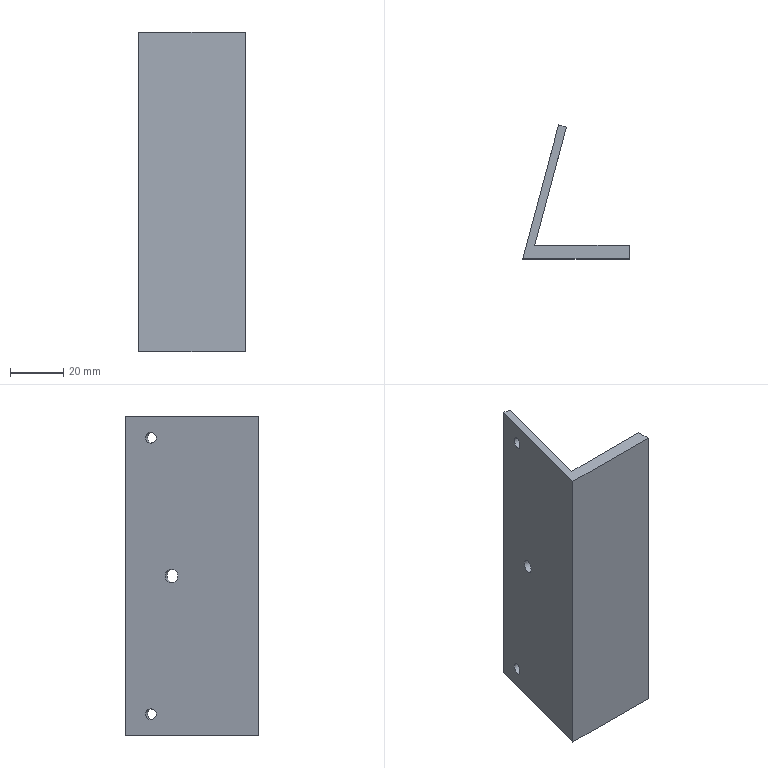Part | NX | features DATUM_CSYS 5, SKETCH 4, EXTRUDE 3, OFFSET_REGION 1 | 1 solid | 11 faces | box 40 x 50.228 x 120 mm | volume 40168 mm3 | plane 8 | cylinder 3 | commonest cylinder face diameters 4.2 x2 5 x1
STEP:
#1=CARTESIAN_POINT('',(0.,0.,-60.));
#2=VERTEX_POINT('',#1);
#3=CARTESIAN_POINT('',(40.,0.,-60.));
#4=VERTEX_POINT('',#3);
#5=CARTESIAN_POINT('',(5.176,0.,-60.));
#6=DIRECTION('',(1.,0.,0.));
#7=VECTOR('',#6,1000.);
#8=LINE('',#5,#7);
#9=EDGE_CURVE('',#2,#4,#8,.T.);
#10=ORIENTED_EDGE('',*,*,#9,.T.);
#11=CARTESIAN_POINT('',(40.,0.,60.));
#12=VERTEX_POINT('',#11);
#13=CARTESIAN_POINT('',(40.,0.,60.));
#14=DIRECTION('',(0.,0.,-1.));
#15=VECTOR('',#14,1000.);
#16=LINE('',#13,#15);
#17=EDGE_CURVE('',#12,#4,#16,.T.);
#18=ORIENTED_EDGE('',*,*,#17,.F.);
#19=CARTESIAN_POINT('',(0.,0.,60.));
#20=VERTEX_POINT('',#19);
#21=CARTESIAN_POINT('',(0.,0.,60.));
#22=DIRECTION('',(1.,0.,0.));
#23=VECTOR('',#22,1000.);
#24=LINE('',#21,#23);
#25=EDGE_CURVE('',#20,#12,#24,.T.);
#26=ORIENTED_EDGE('',*,*,#25,.F.);
#27=CARTESIAN_POINT('',(0.,0.,60.));
#28=DIRECTION('',(0.,0.,-1.));
#29=VECTOR('',#28,1000.);
#30=LINE('',#27,#29);
#31=EDGE_CURVE('',#20,#2,#30,.T.);
#32=ORIENTED_EDGE('',*,*,#31,.T.);
#33=EDGE_LOOP('',(#10,#18,#26,#32));
#34=FACE_BOUND('',#33,.T.);
#35=CARTESIAN_POINT('',(5.176,0.,60.));
#36=DIRECTION('',(0.,1.,0.));
#37=DIRECTION('',(0.,0.,1.));
#38=AXIS2_PLACEMENT_3D('',#35,#36,#37);
#39=PLANE('',#38);
#40=ADVANCED_FACE('',(#34),#39,.F.);
#41=CARTESIAN_POINT('',(40.,5.,-60.));
#42=VERTEX_POINT('',#41);
#43=CARTESIAN_POINT('',(40.,0.,-60.));
#44=DIRECTION('',(0.,1.,0.));
#45=VECTOR('',#44,1000.);
#46=LINE('',#43,#45);
#47=EDGE_CURVE('',#4,#42,#46,.T.);
#48=ORIENTED_EDGE('',*,*,#47,.T.);
#49=CARTESIAN_POINT('',(40.,5.,60.));
#50=VERTEX_POINT('',#49);
#51=CARTESIAN_POINT('',(40.,5.,60.));
#52=DIRECTION('',(0.,0.,-1.));
#53=VECTOR('',#52,1000.);
#54=LINE('',#51,#53);
#55=EDGE_CURVE('',#50,#42,#54,.T.);
#56=ORIENTED_EDGE('',*,*,#55,.F.);
#57=CARTESIAN_POINT('',(40.,0.,60.));
#58=DIRECTION('',(0.,1.,0.));
#59=VECTOR('',#58,1000.);
#60=LINE('',#57,#59);
#61=EDGE_CURVE('',#12,#50,#60,.T.);
#62=ORIENTED_EDGE('',*,*,#61,.F.);
#63=ORIENTED_EDGE('',*,*,#17,.T.);
#64=EDGE_LOOP('',(#48,#56,#62,#63));
#65=FACE_BOUND('',#64,.T.);
#66=CARTESIAN_POINT('',(40.,0.,60.));
#67=DIRECTION('',(-1.,0.,0.));
#68=DIRECTION('',(0.,0.,1.));
#69=AXIS2_PLACEMENT_3D('',#66,#67,#68);
#70=PLANE('',#69);
#71=ADVANCED_FACE('',(#65),#70,.F.);
#72=CARTESIAN_POINT('',(4.446,5.,-60.));
#73=VERTEX_POINT('',#72);
#74=CARTESIAN_POINT('',(40.,5.,-60.));
#75=DIRECTION('',(-1.,0.,0.));
#76=VECTOR('',#75,1000.);
#77=LINE('',#74,#76);
#78=EDGE_CURVE('',#42,#73,#77,.T.);
#79=ORIENTED_EDGE('',*,*,#78,.T.);
#80=CARTESIAN_POINT('',(4.446,5.,60.));
#81=VERTEX_POINT('',#80);
#82=CARTESIAN_POINT('',(4.446,5.,60.));
#83=DIRECTION('',(0.,0.,-1.));
#84=VECTOR('',#83,1000.);
#85=LINE('',#82,#84);
#86=EDGE_CURVE('',#81,#73,#85,.T.);
#87=ORIENTED_EDGE('',*,*,#86,.F.);
#88=CARTESIAN_POINT('',(40.,5.,60.));
#89=DIRECTION('',(-1.,0.,0.));
#90=VECTOR('',#89,1000.);
#91=LINE('',#88,#90);
#92=EDGE_CURVE('',#50,#81,#91,.T.);
#93=ORIENTED_EDGE('',*,*,#92,.F.);
#94=ORIENTED_EDGE('',*,*,#55,.T.);
#95=EDGE_LOOP('',(#79,#87,#93,#94));
#96=FACE_BOUND('',#95,.T.);
#97=CARTESIAN_POINT('',(40.,5.,60.));
#98=DIRECTION('',(0.,-1.,0.));
#99=DIRECTION('',(0.,0.,-1.));
#100=AXIS2_PLACEMENT_3D('',#97,#98,#99);
#101=PLANE('',#100);
#102=ADVANCED_FACE('',(#96),#101,.F.);
#103=CARTESIAN_POINT('',(11.051,29.65,0.));
#104=VERTEX_POINT('',#103);
#105=CARTESIAN_POINT('',(11.698,32.065,0.));
#106=DIRECTION('',(-0.9659,0.2588,0.));
#107=DIRECTION('',(-0.2588,-0.9659,0.));
#108=AXIS2_PLACEMENT_3D('',#105,#106,#107);
#109=CIRCLE('',#108,2.5);
#110=EDGE_CURVE('',#104,#104,#109,.F.);
#111=ORIENTED_EDGE('',*,*,#110,.F.);
#112=EDGE_LOOP('',(#111));
#113=FACE_BOUND('',#112,.T.);
#114=CARTESIAN_POINT('',(13.225,37.764,-52.));
#115=VERTEX_POINT('',#114);
#116=CARTESIAN_POINT('',(13.768,39.792,-52.));
#117=DIRECTION('',(-0.9659,0.2588,0.));
#118=DIRECTION('',(-0.2588,-0.9659,0.));
#119=AXIS2_PLACEMENT_3D('',#116,#117,#118);
#120=CIRCLE('',#119,2.1);
#121=EDGE_CURVE('',#115,#115,#120,.F.);
#122=ORIENTED_EDGE('',*,*,#121,.F.);
#123=EDGE_LOOP('',(#122));
#124=FACE_BOUND('',#123,.T.);
#125=CARTESIAN_POINT('',(13.225,37.764,52.));
#126=VERTEX_POINT('',#125);
#127=CARTESIAN_POINT('',(13.768,39.792,52.));
#128=DIRECTION('',(-0.9659,0.2588,0.));
#129=DIRECTION('',(-0.2588,-0.9659,0.));
#130=AXIS2_PLACEMENT_3D('',#127,#128,#129);
#131=CIRCLE('',#130,2.1);
#132=EDGE_CURVE('',#126,#126,#131,.F.);
#133=ORIENTED_EDGE('',*,*,#132,.F.);
#134=EDGE_LOOP('',(#133));
#135=FACE_BOUND('',#134,.T.);
#136=CARTESIAN_POINT('',(16.356,49.452,-60.));
#137=VERTEX_POINT('',#136);
#138=CARTESIAN_POINT('',(4.584,5.518,-60.));
#139=DIRECTION('',(0.2588,0.9659,0.));
#140=VECTOR('',#139,1000.);
#141=LINE('',#138,#140);
#142=EDGE_CURVE('',#73,#137,#141,.T.);
#143=ORIENTED_EDGE('',*,*,#142,.T.);
#144=CARTESIAN_POINT('',(16.356,49.452,60.));
#145=VERTEX_POINT('',#144);
#146=CARTESIAN_POINT('',(16.356,49.452,60.));
#147=DIRECTION('',(0.,0.,-1.));
#148=VECTOR('',#147,1000.);
#149=LINE('',#146,#148);
#150=EDGE_CURVE('',#145,#137,#149,.T.);
#151=ORIENTED_EDGE('',*,*,#150,.F.);
#152=CARTESIAN_POINT('',(4.584,5.518,60.));
#153=DIRECTION('',(0.2588,0.9659,0.));
#154=VECTOR('',#153,1000.);
#155=LINE('',#152,#154);
#156=EDGE_CURVE('',#81,#145,#155,.T.);
#157=ORIENTED_EDGE('',*,*,#156,.F.);
#158=ORIENTED_EDGE('',*,*,#86,.T.);
#159=EDGE_LOOP('',(#143,#151,#157,#158));
#160=FACE_BOUND('',#159,.T.);
#161=CARTESIAN_POINT('',(4.584,5.518,60.));
#162=DIRECTION('',(-0.9659,0.2588,0.));
#163=DIRECTION('',(-0.2588,-0.9659,0.));
#164=AXIS2_PLACEMENT_3D('',#161,#162,#163);
#165=PLANE('',#164);
#166=ADVANCED_FACE('',(#113,#124,#135,#160),#165,.F.);
#167=CARTESIAN_POINT('',(13.459,50.228,-60.));
#168=VERTEX_POINT('',#167);
#169=CARTESIAN_POINT('',(18.288,48.934,-60.));
#170=DIRECTION('',(-0.9659,0.2588,0.));
#171=VECTOR('',#170,1000.);
#172=LINE('',#169,#171);
#173=EDGE_CURVE('',#137,#168,#172,.T.);
#174=ORIENTED_EDGE('',*,*,#173,.T.);
#175=CARTESIAN_POINT('',(13.459,50.228,60.));
#176=VERTEX_POINT('',#175);
#177=CARTESIAN_POINT('',(13.459,50.228,60.));
#178=DIRECTION('',(0.,0.,-1.));
#179=VECTOR('',#178,1000.);
#180=LINE('',#177,#179);
#181=EDGE_CURVE('',#176,#168,#180,.T.);
#182=ORIENTED_EDGE('',*,*,#181,.F.);
#183=CARTESIAN_POINT('',(18.288,48.934,60.));
#184=DIRECTION('',(-0.9659,0.2588,0.));
#185=VECTOR('',#184,1000.);
#186=LINE('',#183,#185);
#187=EDGE_CURVE('',#145,#176,#186,.T.);
#188=ORIENTED_EDGE('',*,*,#187,.F.);
#189=ORIENTED_EDGE('',*,*,#150,.T.);
#190=EDGE_LOOP('',(#174,#182,#188,#189));
#191=FACE_BOUND('',#190,.T.);
#192=CARTESIAN_POINT('',(18.288,48.934,60.));
#193=DIRECTION('',(-0.2588,-0.9659,0.));
#194=DIRECTION('',(0.9659,-0.2588,0.));
#195=AXIS2_PLACEMENT_3D('',#192,#193,#194);
#196=PLANE('',#195);
#197=ADVANCED_FACE('',(#191),#196,.F.);
#198=CARTESIAN_POINT('',(9.447,35.256,0.));
#199=VERTEX_POINT('',#198);
#200=CARTESIAN_POINT('',(8.8,32.841,0.));
#201=DIRECTION('',(0.9659,-0.2588,0.));
#202=DIRECTION('',(0.2588,0.9659,0.));
#203=AXIS2_PLACEMENT_3D('',#200,#201,#202);
#204=CIRCLE('',#203,2.5);
#205=EDGE_CURVE('',#199,#199,#204,.F.);
#206=ORIENTED_EDGE('',*,*,#205,.F.);
#207=EDGE_LOOP('',(#206));
#208=FACE_BOUND('',#207,.T.);
#209=CARTESIAN_POINT('',(11.414,42.597,-52.));
#210=VERTEX_POINT('',#209);
#211=CARTESIAN_POINT('',(10.87,40.569,-52.));
#212=DIRECTION('',(0.9659,-0.2588,0.));
#213=DIRECTION('',(0.2588,0.9659,0.));
#214=AXIS2_PLACEMENT_3D('',#211,#212,#213);
#215=CIRCLE('',#214,2.1);
#216=EDGE_CURVE('',#210,#210,#215,.F.);
#217=ORIENTED_EDGE('',*,*,#216,.F.);
#218=EDGE_LOOP('',(#217));
#219=FACE_BOUND('',#218,.T.);
#220=CARTESIAN_POINT('',(11.414,42.597,52.));
#221=VERTEX_POINT('',#220);
#222=CARTESIAN_POINT('',(10.87,40.569,52.));
#223=DIRECTION('',(0.9659,-0.2588,0.));
#224=DIRECTION('',(0.2588,0.9659,0.));
#225=AXIS2_PLACEMENT_3D('',#222,#223,#224);
#226=CIRCLE('',#225,2.1);
#227=EDGE_CURVE('',#221,#221,#226,.F.);
#228=ORIENTED_EDGE('',*,*,#227,.F.);
#229=EDGE_LOOP('',(#228));
#230=FACE_BOUND('',#229,.T.);
#231=CARTESIAN_POINT('',(13.459,50.228,-60.));
#232=DIRECTION('',(-0.2588,-0.9659,0.));
#233=VECTOR('',#232,1000.);
#234=LINE('',#231,#233);
#235=EDGE_CURVE('',#168,#2,#234,.T.);
#236=ORIENTED_EDGE('',*,*,#235,.T.);
#237=ORIENTED_EDGE('',*,*,#31,.F.);
#238=CARTESIAN_POINT('',(13.459,50.228,60.));
#239=DIRECTION('',(-0.2588,-0.9659,0.));
#240=VECTOR('',#239,1000.);
#241=LINE('',#238,#240);
#242=EDGE_CURVE('',#176,#20,#241,.T.);
#243=ORIENTED_EDGE('',*,*,#242,.F.);
#244=ORIENTED_EDGE('',*,*,#181,.T.);
#245=EDGE_LOOP('',(#236,#237,#243,#244));
#246=FACE_BOUND('',#245,.T.);
#247=CARTESIAN_POINT('',(13.459,50.228,60.));
#248=DIRECTION('',(0.9659,-0.2588,0.));
#249=DIRECTION('',(0.2588,0.9659,0.));
#250=AXIS2_PLACEMENT_3D('',#247,#248,#249);
#251=PLANE('',#250);
#252=ADVANCED_FACE('',(#208,#219,#230,#246),#251,.F.);
#253=ORIENTED_EDGE('',*,*,#25,.T.);
#254=ORIENTED_EDGE('',*,*,#61,.T.);
#255=ORIENTED_EDGE('',*,*,#92,.T.);
#256=ORIENTED_EDGE('',*,*,#156,.T.);
#257=ORIENTED_EDGE('',*,*,#187,.T.);
#258=ORIENTED_EDGE('',*,*,#242,.T.);
#259=EDGE_LOOP('',(#253,#254,#255,#256,#257,#258));
#260=FACE_BOUND('',#259,.T.);
#261=CARTESIAN_POINT('',(0.,0.,60.));
#262=DIRECTION('',(0.,0.,1.));
#263=DIRECTION('',(1.,0.,0.));
#264=AXIS2_PLACEMENT_3D('',#261,#262,#263);
#265=PLANE('',#264);
#266=ADVANCED_FACE('',(#260),#265,.T.);
#267=ORIENTED_EDGE('',*,*,#9,.F.);
#268=ORIENTED_EDGE('',*,*,#235,.F.);
#269=ORIENTED_EDGE('',*,*,#173,.F.);
#270=ORIENTED_EDGE('',*,*,#142,.F.);
#271=ORIENTED_EDGE('',*,*,#78,.F.);
#272=ORIENTED_EDGE('',*,*,#47,.F.);
#273=EDGE_LOOP('',(#267,#268,#269,#270,#271,#272));
#274=FACE_BOUND('',#273,.T.);
#275=CARTESIAN_POINT('',(0.,0.,-60.));
#276=DIRECTION('',(0.,0.,1.));
#277=DIRECTION('',(1.,0.,0.));
#278=AXIS2_PLACEMENT_3D('',#275,#276,#277);
#279=PLANE('',#278);
#280=ADVANCED_FACE('',(#274),#279,.F.);
#281=ORIENTED_EDGE('',*,*,#227,.T.);
#282=EDGE_LOOP('',(#281));
#283=FACE_BOUND('',#282,.T.);
#284=ORIENTED_EDGE('',*,*,#132,.T.);
#285=EDGE_LOOP('',(#284));
#286=FACE_BOUND('',#285,.T.);
#287=CARTESIAN_POINT('',(1.211,43.157,52.));
#288=DIRECTION('',(0.9659,-0.2588,0.));
#289=DIRECTION('',(0.2588,0.9659,0.));
#290=AXIS2_PLACEMENT_3D('',#287,#288,#289);
#291=CYLINDRICAL_SURFACE('',#290,2.1);
#292=ADVANCED_FACE('',(#283,#286),#291,.F.);
#293=ORIENTED_EDGE('',*,*,#216,.T.);
#294=EDGE_LOOP('',(#293));
#295=FACE_BOUND('',#294,.T.);
#296=ORIENTED_EDGE('',*,*,#121,.T.);
#297=EDGE_LOOP('',(#296));
#298=FACE_BOUND('',#297,.T.);
#299=CARTESIAN_POINT('',(1.211,43.157,-52.));
#300=DIRECTION('',(0.9659,-0.2588,0.));
#301=DIRECTION('',(0.2588,0.9659,0.));
#302=AXIS2_PLACEMENT_3D('',#299,#300,#301);
#303=CYLINDRICAL_SURFACE('',#302,2.1);
#304=ADVANCED_FACE('',(#295,#298),#303,.F.);
#305=ORIENTED_EDGE('',*,*,#205,.T.);
#306=EDGE_LOOP('',(#305));
#307=FACE_BOUND('',#306,.T.);
#308=ORIENTED_EDGE('',*,*,#110,.T.);
#309=EDGE_LOOP('',(#308));
#310=FACE_BOUND('',#309,.T.);
#311=CARTESIAN_POINT('',(3.97,34.136,0.));
#312=DIRECTION('',(0.9659,-0.2588,0.));
#313=DIRECTION('',(0.2588,0.9659,0.));
#314=AXIS2_PLACEMENT_3D('',#311,#312,#313);
#315=CYLINDRICAL_SURFACE('',#314,2.5);
#316=ADVANCED_FACE('',(#307,#310),#315,.F.);
#317=CLOSED_SHELL('',(#40,#71,#102,#166,#197,#252,#266,#280,#292,#304,#316));
#318=MANIFOLD_SOLID_BREP('',#317);
#319=(LENGTH_UNIT()NAMED_UNIT(*)SI_UNIT(.MILLI.,.METRE.));
#320=UNCERTAINTY_MEASURE_WITH_UNIT(LENGTH_MEASURE(0.00001),#319,'','');
#321=(NAMED_UNIT(*)PLANE_ANGLE_UNIT()SI_UNIT($,.RADIAN.));
#322=(NAMED_UNIT(*)SI_UNIT($,.STERADIAN.)SOLID_ANGLE_UNIT());
#323=(GEOMETRIC_REPRESENTATION_CONTEXT(3)GLOBAL_UNCERTAINTY_ASSIGNED_CONTEXT((#320))GLOBAL_UNIT_ASSIGNED_CONTEXT((#319,#321,#322))REPRESENTATION_CONTEXT('',''));
#324=ADVANCED_BREP_SHAPE_REPRESENTATION('',(#318),#323);